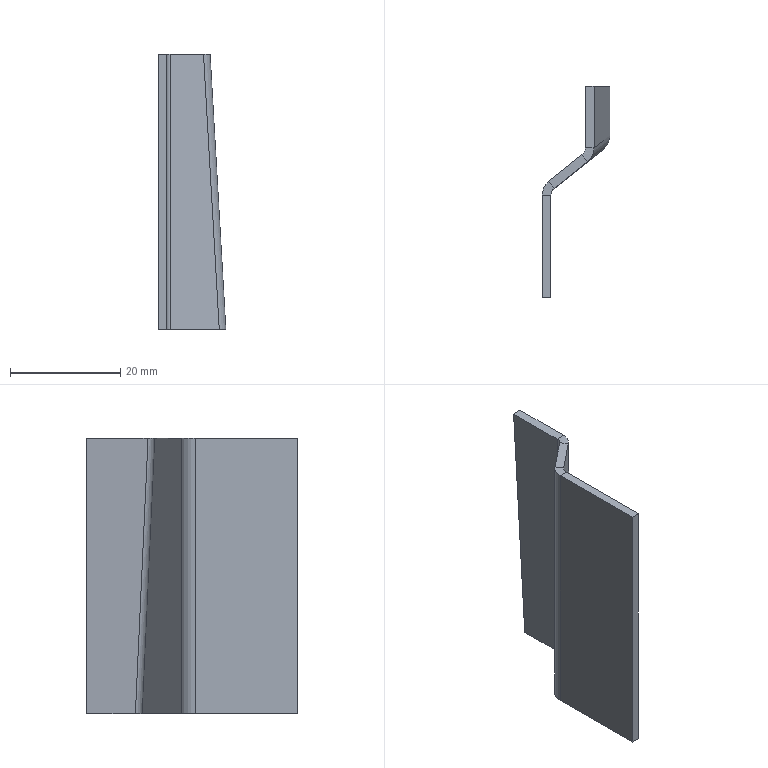Part | SolidWorks | features Fillet 2, Blend 1, FlatPattern 1, SheetMetal 1, SolidToSheetMetal 1 | 1 solid | 22 faces | box 12.3 x 38.3 x 50.091 mm | volume 3396 mm3 | plane 16 | cylinder 4 | spline 2 | commonest cylinder face diameters 3.2 x2 6.4 x2
STEP:
#1=CARTESIAN_POINT('',(9.103,38.3,-50.091));
#2=VERTEX_POINT('',#1);
#3=CARTESIAN_POINT('',(10.7,38.3,-50.));
#4=VERTEX_POINT('',#3);
#5=CARTESIAN_POINT('',(9.103,38.3,-50.091));
#6=CARTESIAN_POINT('',(9.635,38.3,-50.061));
#7=CARTESIAN_POINT('',(10.168,38.3,-50.03));
#8=CARTESIAN_POINT('',(10.7,38.3,-50.));
#9=B_SPLINE_CURVE_WITH_KNOTS('',3,(#5,#6,#7,#8),.UNSPECIFIED.,.F.,.F.,(4,4),(0.,1.),.UNSPECIFIED.);
#10=EDGE_CURVE('',#2,#4,#9,.T.);
#11=ORIENTED_EDGE('',*,*,#10,.F.);
#12=CARTESIAN_POINT('',(6.241,38.3,-0.09142));
#13=VERTEX_POINT('',#12);
#14=CARTESIAN_POINT('',(6.215,38.3,0.3557));
#15=DIRECTION('',(-0.05714,0.,0.9984));
#16=VECTOR('',#15,1000.);
#17=LINE('',#14,#16);
#18=EDGE_CURVE('',#2,#13,#17,.T.);
#19=ORIENTED_EDGE('',*,*,#18,.T.);
#20=CARTESIAN_POINT('',(7.838,38.3,0.));
#21=VERTEX_POINT('',#20);
#22=CARTESIAN_POINT('',(6.241,38.3,-0.09142));
#23=CARTESIAN_POINT('',(6.773,38.3,-0.06095));
#24=CARTESIAN_POINT('',(7.306,38.3,-0.03047));
#25=CARTESIAN_POINT('',(7.838,38.3,0.));
#26=B_SPLINE_CURVE_WITH_KNOTS('',3,(#22,#23,#24,#25),.UNSPECIFIED.,.F.,.F.,(4,4),(0.,1.),.UNSPECIFIED.);
#27=EDGE_CURVE('',#13,#21,#26,.T.);
#28=ORIENTED_EDGE('',*,*,#27,.T.);
#29=CARTESIAN_POINT('',(10.7,38.3,-50.));
#30=DIRECTION('',(-0.05714,0.,0.9984));
#31=VECTOR('',#30,1000.);
#32=LINE('',#29,#31);
#33=EDGE_CURVE('',#4,#21,#32,.T.);
#34=ORIENTED_EDGE('',*,*,#33,.F.);
#35=EDGE_LOOP('',(#11,#19,#28,#34));
#36=FACE_OUTER_BOUND('',#35,.T.);
#37=CARTESIAN_POINT('',(10.7,38.3,-50.));
#38=DIRECTION('',(0.,-1.,0.));
#39=DIRECTION('',(-0.05714,0.,0.9984));
#40=AXIS2_PLACEMENT_3D('',#37,#38,#39);
#41=PLANE('',#40);
#42=ADVANCED_FACE('',(#36),#41,.F.);
#43=ORIENTED_EDGE('',*,*,#27,.F.);
#44=CARTESIAN_POINT('',(6.241,27.138,-0.09142));
#45=VERTEX_POINT('',#44);
#46=CARTESIAN_POINT('',(6.241,27.138,-0.09142));
#47=CARTESIAN_POINT('',(6.241,30.858,-0.09142));
#48=CARTESIAN_POINT('',(6.241,34.579,-0.09142));
#49=CARTESIAN_POINT('',(6.241,38.3,-0.09142));
#50=B_SPLINE_CURVE_WITH_KNOTS('',3,(#46,#47,#48,#49),.UNSPECIFIED.,.F.,.F.,(4,4),(0.0000024,0.8789),.UNSPECIFIED.);
#51=EDGE_CURVE('',#45,#13,#50,.T.);
#52=ORIENTED_EDGE('',*,*,#51,.F.);
#53=CARTESIAN_POINT('',(7.838,27.138,0.));
#54=VERTEX_POINT('',#53);
#55=CARTESIAN_POINT('',(6.241,27.138,-0.09142));
#56=CARTESIAN_POINT('',(6.773,27.138,-0.06095));
#57=CARTESIAN_POINT('',(7.306,27.138,-0.03047));
#58=CARTESIAN_POINT('',(7.838,27.138,0.));
#59=B_SPLINE_CURVE_WITH_KNOTS('',3,(#55,#56,#57,#58),.UNSPECIFIED.,.F.,.F.,(4,4),(0.,1.),.UNSPECIFIED.);
#60=EDGE_CURVE('',#45,#54,#59,.T.);
#61=ORIENTED_EDGE('',*,*,#60,.T.);
#62=CARTESIAN_POINT('',(7.838,25.6,0.));
#63=DIRECTION('',(0.,1.,0.));
#64=VECTOR('',#63,1000.);
#65=LINE('',#62,#64);
#66=EDGE_CURVE('',#54,#21,#65,.T.);
#67=ORIENTED_EDGE('',*,*,#66,.T.);
#68=EDGE_LOOP('',(#43,#52,#61,#67));
#69=FACE_OUTER_BOUND('',#68,.T.);
#70=CARTESIAN_POINT('',(6.241,38.3,-0.09142));
#71=DIRECTION('',(0.05714,0.,-0.9984));
#72=DIRECTION('',(0.9984,0.,0.05714));
#73=AXIS2_PLACEMENT_3D('',#70,#71,#72);
#74=PLANE('',#73);
#75=ADVANCED_FACE('',(#69),#74,.F.);
#76=ORIENTED_EDGE('',*,*,#60,.F.);
#77=CARTESIAN_POINT('',(5.635,25.882,0.));
#78=VERTEX_POINT('',#77);
#79=CARTESIAN_POINT('',(5.635,25.882,0.));
#80=CARTESIAN_POINT('',(6.024,26.194,-0.03618));
#81=CARTESIAN_POINT('',(6.24,26.642,-0.06879));
#82=CARTESIAN_POINT('',(6.241,27.138,-0.09142));
#83=(BOUNDED_CURVE()B_SPLINE_CURVE(3,(#79,#80,#81,#82),.UNSPECIFIED.,.F.,.F.)B_SPLINE_CURVE_WITH_KNOTS((4,4),(1.571,2.466),.UNSPECIFIED.)CURVE()GEOMETRIC_REPRESENTATION_ITEM()RATIONAL_B_SPLINE_CURVE((1.,0.9343,0.9343,1.))REPRESENTATION_ITEM(''));
#84=EDGE_CURVE('',#78,#45,#83,.T.);
#85=ORIENTED_EDGE('',*,*,#84,.F.);
#86=CARTESIAN_POINT('',(6.638,24.635,0.));
#87=VERTEX_POINT('',#86);
#88=CARTESIAN_POINT('',(5.635,25.882,0.));
#89=CARTESIAN_POINT('',(5.97,25.466,0.));
#90=CARTESIAN_POINT('',(6.304,25.051,0.));
#91=CARTESIAN_POINT('',(6.638,24.635,0.));
#92=(BOUNDED_CURVE()B_SPLINE_CURVE(3,(#88,#89,#90,#91),.UNSPECIFIED.,.F.,.F.)B_SPLINE_CURVE_WITH_KNOTS((4,4),(0.,1.),.UNSPECIFIED.)CURVE()GEOMETRIC_REPRESENTATION_ITEM()RATIONAL_B_SPLINE_CURVE((0.5,0.5,0.5,0.5))REPRESENTATION_ITEM(''));
#93=EDGE_CURVE('',#78,#87,#92,.T.);
#94=ORIENTED_EDGE('',*,*,#93,.T.);
#95=CARTESIAN_POINT('',(6.638,24.635,0.));
#96=CARTESIAN_POINT('',(7.41,25.256,0.));
#97=CARTESIAN_POINT('',(7.838,26.149,0.));
#98=CARTESIAN_POINT('',(7.838,27.138,0.));
#99=(BOUNDED_CURVE()B_SPLINE_CURVE(3,(#95,#96,#97,#98),.UNSPECIFIED.,.F.,.F.)B_SPLINE_CURVE_WITH_KNOTS((4,4),(1.571,2.466),.UNSPECIFIED.)CURVE()GEOMETRIC_REPRESENTATION_ITEM()RATIONAL_B_SPLINE_CURVE((1.,0.9343,0.9343,1.))REPRESENTATION_ITEM(''));
#100=EDGE_CURVE('',#87,#54,#99,.T.);
#101=ORIENTED_EDGE('',*,*,#100,.T.);
#102=EDGE_LOOP('',(#76,#85,#94,#101));
#103=FACE_OUTER_BOUND('',#102,.T.);
#104=CARTESIAN_POINT('',(3.376,26.119,0.1172));
#105=CARTESIAN_POINT('',(2.961,25.786,0.07811));
#106=CARTESIAN_POINT('',(2.547,25.452,0.03906));
#107=CARTESIAN_POINT('',(2.132,25.119,0.));
#108=CARTESIAN_POINT('',(5.381,23.625,0.1172));
#109=CARTESIAN_POINT('',(5.634,22.46,0.07811));
#110=CARTESIAN_POINT('',(5.888,21.295,0.03906));
#111=CARTESIAN_POINT('',(6.142,20.131,0.));
#112=CARTESIAN_POINT('',(7.895,25.646,-0.1172));
#113=CARTESIAN_POINT('',(8.978,25.147,-0.07811));
#114=CARTESIAN_POINT('',(10.061,24.649,-0.03906));
#115=CARTESIAN_POINT('',(11.143,24.151,0.));
#116=CARTESIAN_POINT('',(5.89,28.14,-0.1172));
#117=CARTESIAN_POINT('',(6.305,28.473,-0.07811));
#118=CARTESIAN_POINT('',(6.719,28.806,-0.03906));
#119=CARTESIAN_POINT('',(7.134,29.139,0.));
#120=CARTESIAN_POINT('',(3.886,30.634,-0.1172));
#121=CARTESIAN_POINT('',(3.632,31.799,-0.07811));
#122=CARTESIAN_POINT('',(3.378,32.963,-0.03906));
#123=CARTESIAN_POINT('',(3.125,34.128,0.));
#124=CARTESIAN_POINT('',(1.371,28.613,0.1172));
#125=CARTESIAN_POINT('',(0.2884,29.111,0.07811));
#126=CARTESIAN_POINT('',(-0.7944,29.609,0.03906));
#127=CARTESIAN_POINT('',(-1.877,30.108,0.));
#128=CARTESIAN_POINT('',(3.376,26.119,0.1172));
#129=CARTESIAN_POINT('',(2.961,25.786,0.07811));
#130=CARTESIAN_POINT('',(2.547,25.452,0.03906));
#131=CARTESIAN_POINT('',(2.132,25.119,0.));
#132=(BOUNDED_SURFACE()B_SPLINE_SURFACE(3,3,((#104,#105,#106,#107),(#108,#109,#110,#111),(#112,#113,#114,#115),(#116,#117,#118,#119),(#120,#121,#122,#123),(#124,#125,#126,#127),(#128,#129,#130,#131)),.UNSPECIFIED.,.T.,.F.,.F.)B_SPLINE_SURFACE_WITH_KNOTS((4,3,4),(4,4),(0.,0.5,1.),(0.,1.),.UNSPECIFIED.)GEOMETRIC_REPRESENTATION_ITEM()RATIONAL_B_SPLINE_SURFACE(((1.,1.,1.,1.),(0.3333,0.3333,0.3333,0.3333),(0.3333,0.3333,0.3333,0.3333),(1.,1.,1.,1.),(0.3333,0.3333,0.3333,0.3333),(0.3333,0.3333,0.3333,0.3333),(1.,1.,1.,1.)))REPRESENTATION_ITEM('')SURFACE());
#133=ADVANCED_FACE('',(#103),#132,.F.);
#134=ORIENTED_EDGE('',*,*,#93,.F.);
#135=CARTESIAN_POINT('',(-0.4047,21.027,0.));
#136=VERTEX_POINT('',#135);
#137=CARTESIAN_POINT('',(-0.4047,21.027,0.));
#138=CARTESIAN_POINT('',(1.609,22.646,0.));
#139=CARTESIAN_POINT('',(3.622,24.264,0.));
#140=CARTESIAN_POINT('',(5.635,25.882,0.));
#141=B_SPLINE_CURVE_WITH_KNOTS('',3,(#137,#138,#139,#140),.UNSPECIFIED.,.F.,.F.,(4,4),(0.1532,0.9238),.UNSPECIFIED.);
#142=EDGE_CURVE('',#136,#78,#141,.T.);
#143=ORIENTED_EDGE('',*,*,#142,.F.);
#144=CARTESIAN_POINT('',(0.5976,19.78,0.));
#145=VERTEX_POINT('',#144);
#146=CARTESIAN_POINT('',(-0.4047,21.027,0.));
#147=CARTESIAN_POINT('',(-0.07059,20.612,0.));
#148=CARTESIAN_POINT('',(0.2635,20.196,0.));
#149=CARTESIAN_POINT('',(0.5976,19.78,0.));
#150=B_SPLINE_CURVE_WITH_KNOTS('',3,(#146,#147,#148,#149),.UNSPECIFIED.,.F.,.F.,(4,4),(0.,1.),.UNSPECIFIED.);
#151=EDGE_CURVE('',#136,#145,#150,.T.);
#152=ORIENTED_EDGE('',*,*,#151,.T.);
#153=CARTESIAN_POINT('',(0.,19.3,0.));
#154=DIRECTION('',(0.7794,0.6265,0.));
#155=VECTOR('',#154,1000.);
#156=LINE('',#153,#155);
#157=EDGE_CURVE('',#145,#87,#156,.T.);
#158=ORIENTED_EDGE('',*,*,#157,.T.);
#159=EDGE_LOOP('',(#134,#143,#152,#158));
#160=FACE_OUTER_BOUND('',#159,.T.);
#161=CARTESIAN_POINT('',(5.635,25.882,0.));
#162=DIRECTION('',(0.,0.,-1.));
#163=DIRECTION('',(0.6265,-0.7794,0.));
#164=AXIS2_PLACEMENT_3D('',#161,#162,#163);
#165=PLANE('',#164);
#166=ADVANCED_FACE('',(#160),#165,.F.);
#167=ORIENTED_EDGE('',*,*,#151,.F.);
#168=CARTESIAN_POINT('',(-1.6,18.533,0.));
#169=VERTEX_POINT('',#168);
#170=CARTESIAN_POINT('',(1.6,18.533,0.));
#171=DIRECTION('',(0.,0.,-1.));
#172=DIRECTION('',(-1.,0.,0.));
#173=AXIS2_PLACEMENT_3D('',#170,#171,#172);
#174=CIRCLE('',#173,3.2);
#175=EDGE_CURVE('',#169,#136,#174,.T.);
#176=ORIENTED_EDGE('',*,*,#175,.F.);
#177=CARTESIAN_POINT('',(0.,18.533,0.));
#178=VERTEX_POINT('',#177);
#179=CARTESIAN_POINT('',(-1.6,18.533,0.));
#180=CARTESIAN_POINT('',(-1.067,18.533,0.));
#181=CARTESIAN_POINT('',(-0.5333,18.533,0.));
#182=CARTESIAN_POINT('',(0.,18.533,0.));
#183=B_SPLINE_CURVE_WITH_KNOTS('',3,(#179,#180,#181,#182),.UNSPECIFIED.,.F.,.F.,(4,4),(0.,1.),.UNSPECIFIED.);
#184=EDGE_CURVE('',#169,#178,#183,.T.);
#185=ORIENTED_EDGE('',*,*,#184,.T.);
#186=CARTESIAN_POINT('',(1.6,18.533,0.));
#187=DIRECTION('',(0.,0.,-1.));
#188=DIRECTION('',(1.,0.,0.));
#189=AXIS2_PLACEMENT_3D('',#186,#187,#188);
#190=CIRCLE('',#189,1.6);
#191=EDGE_CURVE('',#178,#145,#190,.T.);
#192=ORIENTED_EDGE('',*,*,#191,.T.);
#193=EDGE_LOOP('',(#167,#176,#185,#192));
#194=FACE_OUTER_BOUND('',#193,.T.);
#195=CARTESIAN_POINT('',(1.6,18.533,0.));
#196=DIRECTION('',(0.,0.,-1.));
#197=DIRECTION('',(-1.,0.,0.));
#198=AXIS2_PLACEMENT_3D('',#195,#196,#197);
#199=PLANE('',#198);
#200=ADVANCED_FACE('',(#194),#199,.F.);
#201=ORIENTED_EDGE('',*,*,#184,.F.);
#202=CARTESIAN_POINT('',(-1.6,0.,0.));
#203=VERTEX_POINT('',#202);
#204=CARTESIAN_POINT('',(-1.6,0.,0.));
#205=CARTESIAN_POINT('',(-1.6,6.178,0.));
#206=CARTESIAN_POINT('',(-1.6,12.355,0.));
#207=CARTESIAN_POINT('',(-1.6,18.533,0.));
#208=B_SPLINE_CURVE_WITH_KNOTS('',3,(#204,#205,#206,#207),.UNSPECIFIED.,.F.,.F.,(4,4),(0.03973,1.),.UNSPECIFIED.);
#209=EDGE_CURVE('',#203,#169,#208,.T.);
#210=ORIENTED_EDGE('',*,*,#209,.F.);
#211=CARTESIAN_POINT('',(0.,0.,0.));
#212=VERTEX_POINT('',#211);
#213=CARTESIAN_POINT('',(-1.6,0.,0.));
#214=CARTESIAN_POINT('',(-1.067,0.,0.));
#215=CARTESIAN_POINT('',(-0.5333,0.,0.));
#216=CARTESIAN_POINT('',(0.,0.,0.));
#217=B_SPLINE_CURVE_WITH_KNOTS('',3,(#213,#214,#215,#216),.UNSPECIFIED.,.F.,.F.,(4,4),(0.,1.),.UNSPECIFIED.);
#218=EDGE_CURVE('',#203,#212,#217,.T.);
#219=ORIENTED_EDGE('',*,*,#218,.T.);
#220=CARTESIAN_POINT('',(0.,19.3,0.));
#221=DIRECTION('',(0.,1.,0.));
#222=VECTOR('',#221,1000.);
#223=LINE('',#220,#222);
#224=EDGE_CURVE('',#212,#178,#223,.T.);
#225=ORIENTED_EDGE('',*,*,#224,.T.);
#226=EDGE_LOOP('',(#201,#210,#219,#225));
#227=FACE_OUTER_BOUND('',#226,.T.);
#228=CARTESIAN_POINT('',(-1.6,18.533,0.));
#229=DIRECTION('',(0.,0.,-1.));
#230=DIRECTION('',(1.,0.,0.));
#231=AXIS2_PLACEMENT_3D('',#228,#229,#230);
#232=PLANE('',#231);
#233=ADVANCED_FACE('',(#227),#232,.F.);
#234=ORIENTED_EDGE('',*,*,#218,.F.);
#235=CARTESIAN_POINT('',(-1.6,0.,-50.));
#236=VERTEX_POINT('',#235);
#237=CARTESIAN_POINT('',(-1.6,0.,0.));
#238=DIRECTION('',(0.,0.,1.));
#239=VECTOR('',#238,1000.);
#240=LINE('',#237,#239);
#241=EDGE_CURVE('',#236,#203,#240,.T.);
#242=ORIENTED_EDGE('',*,*,#241,.F.);
#243=CARTESIAN_POINT('',(0.,0.,-50.));
#244=VERTEX_POINT('',#243);
#245=CARTESIAN_POINT('',(-1.6,0.,-50.));
#246=CARTESIAN_POINT('',(-1.067,0.,-50.));
#247=CARTESIAN_POINT('',(-0.5333,0.,-50.));
#248=CARTESIAN_POINT('',(0.,0.,-50.));
#249=B_SPLINE_CURVE_WITH_KNOTS('',3,(#245,#246,#247,#248),.UNSPECIFIED.,.F.,.F.,(4,4),(0.,1.),.UNSPECIFIED.);
#250=EDGE_CURVE('',#236,#244,#249,.T.);
#251=ORIENTED_EDGE('',*,*,#250,.T.);
#252=CARTESIAN_POINT('',(0.,0.,-50.));
#253=DIRECTION('',(0.,0.,1.));
#254=VECTOR('',#253,1000.);
#255=LINE('',#252,#254);
#256=EDGE_CURVE('',#244,#212,#255,.T.);
#257=ORIENTED_EDGE('',*,*,#256,.T.);
#258=EDGE_LOOP('',(#234,#242,#251,#257));
#259=FACE_OUTER_BOUND('',#258,.T.);
#260=CARTESIAN_POINT('',(0.,0.,-50.));
#261=DIRECTION('',(0.,-1.,0.));
#262=DIRECTION('',(0.,0.,1.));
#263=AXIS2_PLACEMENT_3D('',#260,#261,#262);
#264=PLANE('',#263);
#265=ADVANCED_FACE('',(#259),#264,.T.);
#266=ORIENTED_EDGE('',*,*,#250,.F.);
#267=CARTESIAN_POINT('',(-1.6,18.533,-50.));
#268=VERTEX_POINT('',#267);
#269=CARTESIAN_POINT('',(-1.6,0.,-50.));
#270=CARTESIAN_POINT('',(-1.6,6.178,-50.));
#271=CARTESIAN_POINT('',(-1.6,12.355,-50.));
#272=CARTESIAN_POINT('',(-1.6,18.533,-50.));
#273=B_SPLINE_CURVE_WITH_KNOTS('',3,(#269,#270,#271,#272),.UNSPECIFIED.,.F.,.F.,(4,4),(0.,1.),.UNSPECIFIED.);
#274=EDGE_CURVE('',#236,#268,#273,.T.);
#275=ORIENTED_EDGE('',*,*,#274,.T.);
#276=CARTESIAN_POINT('',(0.,18.533,-50.));
#277=VERTEX_POINT('',#276);
#278=CARTESIAN_POINT('',(-1.6,18.533,-50.));
#279=CARTESIAN_POINT('',(-1.067,18.533,-50.));
#280=CARTESIAN_POINT('',(-0.5333,18.533,-50.));
#281=CARTESIAN_POINT('',(0.,18.533,-50.));
#282=B_SPLINE_CURVE_WITH_KNOTS('',3,(#278,#279,#280,#281),.UNSPECIFIED.,.F.,.F.,(4,4),(0.,1.),.UNSPECIFIED.);
#283=EDGE_CURVE('',#268,#277,#282,.T.);
#284=ORIENTED_EDGE('',*,*,#283,.T.);
#285=CARTESIAN_POINT('',(0.,0.,-50.));
#286=DIRECTION('',(0.,1.,0.));
#287=VECTOR('',#286,1000.);
#288=LINE('',#285,#287);
#289=EDGE_CURVE('',#244,#277,#288,.T.);
#290=ORIENTED_EDGE('',*,*,#289,.F.);
#291=EDGE_LOOP('',(#266,#275,#284,#290));
#292=FACE_OUTER_BOUND('',#291,.T.);
#293=CARTESIAN_POINT('',(-1.6,0.,-50.));
#294=DIRECTION('',(0.,0.,1.));
#295=DIRECTION('',(1.,0.,0.));
#296=AXIS2_PLACEMENT_3D('',#293,#294,#295);
#297=PLANE('',#296);
#298=ADVANCED_FACE('',(#292),#297,.F.);
#299=ORIENTED_EDGE('',*,*,#283,.F.);
#300=CARTESIAN_POINT('',(-0.4047,21.027,-50.));
#301=VERTEX_POINT('',#300);
#302=CARTESIAN_POINT('',(1.6,18.533,-50.));
#303=DIRECTION('',(0.,0.,1.));
#304=DIRECTION('',(-1.,0.,0.));
#305=AXIS2_PLACEMENT_3D('',#302,#303,#304);
#306=CIRCLE('',#305,3.2);
#307=EDGE_CURVE('',#301,#268,#306,.T.);
#308=ORIENTED_EDGE('',*,*,#307,.F.);
#309=CARTESIAN_POINT('',(0.5976,19.78,-50.));
#310=VERTEX_POINT('',#309);
#311=CARTESIAN_POINT('',(-0.4047,21.027,-50.));
#312=CARTESIAN_POINT('',(-0.07059,20.612,-50.));
#313=CARTESIAN_POINT('',(0.2635,20.196,-50.));
#314=CARTESIAN_POINT('',(0.5976,19.78,-50.));
#315=B_SPLINE_CURVE_WITH_KNOTS('',3,(#311,#312,#313,#314),.UNSPECIFIED.,.F.,.F.,(4,4),(0.,1.),.UNSPECIFIED.);
#316=EDGE_CURVE('',#301,#310,#315,.T.);
#317=ORIENTED_EDGE('',*,*,#316,.T.);
#318=CARTESIAN_POINT('',(1.6,18.533,-50.));
#319=DIRECTION('',(0.,0.,1.));
#320=DIRECTION('',(1.,0.,0.));
#321=AXIS2_PLACEMENT_3D('',#318,#319,#320);
#322=CIRCLE('',#321,1.6);
#323=EDGE_CURVE('',#310,#277,#322,.T.);
#324=ORIENTED_EDGE('',*,*,#323,.T.);
#325=EDGE_LOOP('',(#299,#308,#317,#324));
#326=FACE_OUTER_BOUND('',#325,.T.);
#327=CARTESIAN_POINT('',(1.6,18.533,-50.));
#328=DIRECTION('',(0.,0.,-1.));
#329=DIRECTION('',(-1.,0.,0.));
#330=AXIS2_PLACEMENT_3D('',#327,#328,#329);
#331=PLANE('',#330);
#332=ADVANCED_FACE('',(#326),#331,.T.);
#333=ORIENTED_EDGE('',*,*,#316,.F.);
#334=CARTESIAN_POINT('',(8.497,28.182,-50.));
#335=VERTEX_POINT('',#334);
#336=CARTESIAN_POINT('',(-0.4047,21.027,-50.));
#337=CARTESIAN_POINT('',(2.563,23.412,-50.));
#338=CARTESIAN_POINT('',(5.53,25.797,-50.));
#339=CARTESIAN_POINT('',(8.497,28.182,-50.));
#340=B_SPLINE_CURVE_WITH_KNOTS('',3,(#336,#337,#338,#339),.UNSPECIFIED.,.F.,.F.,(4,4),(0.,1.),.UNSPECIFIED.);
#341=EDGE_CURVE('',#301,#335,#340,.T.);
#342=ORIENTED_EDGE('',*,*,#341,.T.);
#343=CARTESIAN_POINT('',(9.499,26.935,-50.));
#344=VERTEX_POINT('',#343);
#345=CARTESIAN_POINT('',(8.497,28.182,-50.));
#346=CARTESIAN_POINT('',(8.831,27.766,-50.));
#347=CARTESIAN_POINT('',(9.165,27.351,-50.));
#348=CARTESIAN_POINT('',(9.499,26.935,-50.));
#349=B_SPLINE_CURVE_WITH_KNOTS('',3,(#345,#346,#347,#348),.UNSPECIFIED.,.F.,.F.,(4,4),(0.,1.),.UNSPECIFIED.);
#350=EDGE_CURVE('',#335,#344,#349,.T.);
#351=ORIENTED_EDGE('',*,*,#350,.T.);
#352=CARTESIAN_POINT('',(0.,19.3,-50.));
#353=DIRECTION('',(0.7794,0.6265,0.));
#354=VECTOR('',#353,1000.);
#355=LINE('',#352,#354);
#356=EDGE_CURVE('',#310,#344,#355,.T.);
#357=ORIENTED_EDGE('',*,*,#356,.F.);
#358=EDGE_LOOP('',(#333,#342,#351,#357));
#359=FACE_OUTER_BOUND('',#358,.T.);
#360=CARTESIAN_POINT('',(-0.4047,21.027,-50.));
#361=DIRECTION('',(0.,0.,1.));
#362=DIRECTION('',(0.6265,-0.7794,0.));
#363=AXIS2_PLACEMENT_3D('',#360,#361,#362);
#364=PLANE('',#363);
#365=ADVANCED_FACE('',(#359),#364,.F.);
#366=ORIENTED_EDGE('',*,*,#350,.F.);
#367=CARTESIAN_POINT('',(9.103,29.438,-50.091));
#368=VERTEX_POINT('',#367);
#369=CARTESIAN_POINT('',(9.103,29.438,-50.091));
#370=CARTESIAN_POINT('',(9.101,28.942,-50.069));
#371=CARTESIAN_POINT('',(8.885,28.494,-50.036));
#372=CARTESIAN_POINT('',(8.497,28.182,-50.));
#373=(BOUNDED_CURVE()B_SPLINE_CURVE(3,(#369,#370,#371,#372),.UNSPECIFIED.,.F.,.F.)B_SPLINE_CURVE_WITH_KNOTS((4,4),(3.817,4.712),.UNSPECIFIED.)CURVE()GEOMETRIC_REPRESENTATION_ITEM()RATIONAL_B_SPLINE_CURVE((1.,0.9343,0.9343,1.))REPRESENTATION_ITEM(''));
#374=EDGE_CURVE('',#368,#335,#373,.T.);
#375=ORIENTED_EDGE('',*,*,#374,.F.);
#376=CARTESIAN_POINT('',(10.7,29.438,-50.));
#377=VERTEX_POINT('',#376);
#378=CARTESIAN_POINT('',(9.103,29.438,-50.091));
#379=CARTESIAN_POINT('',(9.635,29.438,-50.061));
#380=CARTESIAN_POINT('',(10.168,29.438,-50.03));
#381=CARTESIAN_POINT('',(10.7,29.438,-50.));
#382=(BOUNDED_CURVE()B_SPLINE_CURVE(3,(#378,#379,#380,#381),.UNSPECIFIED.,.F.,.F.)B_SPLINE_CURVE_WITH_KNOTS((4,4),(0.,1.),.UNSPECIFIED.)CURVE()GEOMETRIC_REPRESENTATION_ITEM()RATIONAL_B_SPLINE_CURVE((0.6152,0.6152,0.6152,0.6152))REPRESENTATION_ITEM(''));
#383=EDGE_CURVE('',#368,#377,#382,.T.);
#384=ORIENTED_EDGE('',*,*,#383,.T.);
#385=CARTESIAN_POINT('',(10.7,29.438,-50.));
#386=CARTESIAN_POINT('',(10.7,28.449,-50.));
#387=CARTESIAN_POINT('',(10.272,27.556,-50.));
#388=CARTESIAN_POINT('',(9.499,26.935,-50.));
#389=(BOUNDED_CURVE()B_SPLINE_CURVE(3,(#385,#386,#387,#388),.UNSPECIFIED.,.F.,.F.)B_SPLINE_CURVE_WITH_KNOTS((4,4),(3.817,4.712),.UNSPECIFIED.)CURVE()GEOMETRIC_REPRESENTATION_ITEM()RATIONAL_B_SPLINE_CURVE((1.,0.9343,0.9343,1.))REPRESENTATION_ITEM(''));
#390=EDGE_CURVE('',#377,#344,#389,.T.);
#391=ORIENTED_EDGE('',*,*,#390,.T.);
#392=EDGE_LOOP('',(#366,#375,#384,#391));
#393=FACE_OUTER_BOUND('',#392,.T.);
#394=CARTESIAN_POINT('',(4.994,27.419,-50.));
#395=CARTESIAN_POINT('',(5.408,27.752,-49.961));
#396=CARTESIAN_POINT('',(5.823,28.086,-49.922));
#397=CARTESIAN_POINT('',(6.238,28.419,-49.883));
#398=CARTESIAN_POINT('',(0.9844,32.408,-50.));
#399=CARTESIAN_POINT('',(2.067,31.909,-49.961));
#400=CARTESIAN_POINT('',(3.15,31.411,-49.922));
#401=CARTESIAN_POINT('',(4.233,30.913,-49.883));
#402=CARTESIAN_POINT('',(5.986,36.428,-50.));
#403=CARTESIAN_POINT('',(6.24,35.263,-50.039));
#404=CARTESIAN_POINT('',(6.494,34.099,-50.078));
#405=CARTESIAN_POINT('',(6.747,32.934,-50.117));
#406=CARTESIAN_POINT('',(9.996,31.439,-50.));
#407=CARTESIAN_POINT('',(9.581,31.106,-50.039));
#408=CARTESIAN_POINT('',(9.167,30.773,-50.078));
#409=CARTESIAN_POINT('',(8.752,30.44,-50.117));
#410=CARTESIAN_POINT('',(14.005,26.451,-50.));
#411=CARTESIAN_POINT('',(12.922,26.949,-50.039));
#412=CARTESIAN_POINT('',(11.839,27.447,-50.078));
#413=CARTESIAN_POINT('',(10.757,27.946,-50.117));
#414=CARTESIAN_POINT('',(9.003,22.431,-50.));
#415=CARTESIAN_POINT('',(8.75,23.595,-49.961));
#416=CARTESIAN_POINT('',(8.496,24.76,-49.922));
#417=CARTESIAN_POINT('',(8.242,25.925,-49.883));
#418=CARTESIAN_POINT('',(4.994,27.419,-50.));
#419=CARTESIAN_POINT('',(5.408,27.752,-49.961));
#420=CARTESIAN_POINT('',(5.823,28.086,-49.922));
#421=CARTESIAN_POINT('',(6.238,28.419,-49.883));
#422=(BOUNDED_SURFACE()B_SPLINE_SURFACE(3,3,((#394,#395,#396,#397),(#398,#399,#400,#401),(#402,#403,#404,#405),(#406,#407,#408,#409),(#410,#411,#412,#413),(#414,#415,#416,#417),(#418,#419,#420,#421)),.UNSPECIFIED.,.T.,.F.,.F.)B_SPLINE_SURFACE_WITH_KNOTS((4,3,4),(4,4),(0.,0.5,1.),(0.,1.),.UNSPECIFIED.)GEOMETRIC_REPRESENTATION_ITEM()RATIONAL_B_SPLINE_SURFACE(((1.,1.,1.,1.),(0.3333,0.3333,0.3333,0.3333),(0.3333,0.3333,0.3333,0.3333),(1.,1.,1.,1.),(0.3333,0.3333,0.3333,0.3333),(0.3333,0.3333,0.3333,0.3333),(1.,1.,1.,1.)))REPRESENTATION_ITEM('')SURFACE());
#423=ADVANCED_FACE('',(#393),#422,.T.);
#424=CARTESIAN_POINT('',(9.103,29.438,-50.091));
#425=CARTESIAN_POINT('',(9.103,32.392,-50.091));
#426=CARTESIAN_POINT('',(9.103,35.346,-50.091));
#427=CARTESIAN_POINT('',(9.103,38.3,-50.091));
#428=B_SPLINE_CURVE_WITH_KNOTS('',3,(#424,#425,#426,#427),.UNSPECIFIED.,.F.,.F.,(4,4),(0.,1.),.UNSPECIFIED.);
#429=EDGE_CURVE('',#368,#2,#428,.T.);
#430=ORIENTED_EDGE('',*,*,#429,.T.);
#431=ORIENTED_EDGE('',*,*,#10,.T.);
#432=CARTESIAN_POINT('',(10.7,38.3,-50.));
#433=DIRECTION('',(0.,1.,0.));
#434=VECTOR('',#433,1000.);
#435=LINE('',#432,#434);
#436=EDGE_CURVE('',#377,#4,#435,.T.);
#437=ORIENTED_EDGE('',*,*,#436,.F.);
#438=ORIENTED_EDGE('',*,*,#383,.F.);
#439=EDGE_LOOP('',(#430,#431,#437,#438));
#440=FACE_OUTER_BOUND('',#439,.T.);
#441=CARTESIAN_POINT('',(9.103,29.438,-50.091));
#442=DIRECTION('',(-0.05714,0.,0.9984));
#443=DIRECTION('',(0.9984,0.,0.05714));
#444=AXIS2_PLACEMENT_3D('',#441,#442,#443);
#445=PLANE('',#444);
#446=ADVANCED_FACE('',(#440),#445,.F.);
#447=ORIENTED_EDGE('',*,*,#390,.F.);
#448=CARTESIAN_POINT('',(7.742,27.06,1.688));
#449=DIRECTION('',(0.05708,0.04588,-0.9973));
#450=VECTOR('',#449,1000.);
#451=LINE('',#448,#450);
#452=EDGE_CURVE('',#54,#377,#451,.T.);
#453=ORIENTED_EDGE('',*,*,#452,.F.);
#454=ORIENTED_EDGE('',*,*,#100,.F.);
#455=CARTESIAN_POINT('',(6.552,24.566,1.505));
#456=DIRECTION('',(-0.05708,-0.04588,0.9973));
#457=VECTOR('',#456,1000.);
#458=LINE('',#455,#457);
#459=EDGE_CURVE('',#344,#87,#458,.T.);
#460=ORIENTED_EDGE('',*,*,#459,.F.);
#461=EDGE_LOOP('',(#447,#453,#454,#460));
#462=FACE_OUTER_BOUND('',#461,.T.);
#463=CARTESIAN_POINT('',(4.547,27.06,1.505));
#464=DIRECTION('',(-0.05708,-0.04588,0.9973));
#465=DIRECTION('',(0.9984,0.,0.05714));
#466=AXIS2_PLACEMENT_3D('',#463,#464,#465);
#467=CYLINDRICAL_SURFACE('',#466,3.2);
#468=ADVANCED_FACE('',(#462),#467,.T.);
#469=ORIENTED_EDGE('',*,*,#66,.F.);
#470=ORIENTED_EDGE('',*,*,#452,.T.);
#471=ORIENTED_EDGE('',*,*,#436,.T.);
#472=ORIENTED_EDGE('',*,*,#33,.T.);
#473=EDGE_LOOP('',(#469,#470,#471,#472));
#474=FACE_OUTER_BOUND('',#473,.T.);
#475=CARTESIAN_POINT('',(7.813,0.,0.4471));
#476=DIRECTION('',(-0.9984,0.,-0.05714));
#477=DIRECTION('',(-0.05714,0.,0.9984));
#478=AXIS2_PLACEMENT_3D('',#475,#476,#477);
#479=PLANE('',#478);
#480=ADVANCED_FACE('',(#474),#479,.F.);
#481=ORIENTED_EDGE('',*,*,#323,.F.);
#482=CARTESIAN_POINT('',(0.5976,19.78,-50.));
#483=DIRECTION('',(0.,0.,-1.));
#484=VECTOR('',#483,1000.);
#485=LINE('',#482,#484);
#486=EDGE_CURVE('',#145,#310,#485,.T.);
#487=ORIENTED_EDGE('',*,*,#486,.F.);
#488=ORIENTED_EDGE('',*,*,#191,.F.);
#489=CARTESIAN_POINT('',(0.,18.533,0.));
#490=DIRECTION('',(0.,0.,1.));
#491=VECTOR('',#490,1000.);
#492=LINE('',#489,#491);
#493=EDGE_CURVE('',#277,#178,#492,.T.);
#494=ORIENTED_EDGE('',*,*,#493,.F.);
#495=EDGE_LOOP('',(#481,#487,#488,#494));
#496=FACE_OUTER_BOUND('',#495,.T.);
#497=CARTESIAN_POINT('',(1.6,18.533,0.));
#498=DIRECTION('',(0.,0.,-1.));
#499=DIRECTION('',(-1.,0.,0.));
#500=AXIS2_PLACEMENT_3D('',#497,#498,#499);
#501=CYLINDRICAL_SURFACE('',#500,1.6);
#502=ADVANCED_FACE('',(#496),#501,.F.);
#503=ORIENTED_EDGE('',*,*,#289,.T.);
#504=ORIENTED_EDGE('',*,*,#493,.T.);
#505=ORIENTED_EDGE('',*,*,#224,.F.);
#506=ORIENTED_EDGE('',*,*,#256,.F.);
#507=EDGE_LOOP('',(#503,#504,#505,#506));
#508=FACE_OUTER_BOUND('',#507,.T.);
#509=CARTESIAN_POINT('',(0.,0.,0.));
#510=DIRECTION('',(-1.,0.,0.));
#511=DIRECTION('',(0.,-1.,0.));
#512=AXIS2_PLACEMENT_3D('',#509,#510,#511);
#513=PLANE('',#512);
#514=ADVANCED_FACE('',(#508),#513,.F.);
#515=ORIENTED_EDGE('',*,*,#356,.T.);
#516=ORIENTED_EDGE('',*,*,#459,.T.);
#517=ORIENTED_EDGE('',*,*,#157,.F.);
#518=ORIENTED_EDGE('',*,*,#486,.T.);
#519=EDGE_LOOP('',(#515,#516,#517,#518));
#520=FACE_OUTER_BOUND('',#519,.T.);
#521=CARTESIAN_POINT('',(-9.424,11.725,0.));
#522=DIRECTION('',(-0.6265,0.7794,0.));
#523=DIRECTION('',(-0.7794,-0.6265,0.));
#524=AXIS2_PLACEMENT_3D('',#521,#522,#523);
#525=PLANE('',#524);
#526=ADVANCED_FACE('',(#520),#525,.F.);
#527=ORIENTED_EDGE('',*,*,#374,.T.);
#528=CARTESIAN_POINT('',(5.549,25.813,1.505));
#529=DIRECTION('',(-0.05708,-0.04588,0.9973));
#530=VECTOR('',#529,1000.);
#531=LINE('',#528,#530);
#532=EDGE_CURVE('',#335,#78,#531,.T.);
#533=ORIENTED_EDGE('',*,*,#532,.T.);
#534=ORIENTED_EDGE('',*,*,#84,.T.);
#535=CARTESIAN_POINT('',(6.144,27.06,1.596));
#536=DIRECTION('',(0.05708,0.04588,-0.9973));
#537=VECTOR('',#536,1000.);
#538=LINE('',#535,#537);
#539=EDGE_CURVE('',#45,#368,#538,.T.);
#540=ORIENTED_EDGE('',*,*,#539,.T.);
#541=EDGE_LOOP('',(#527,#533,#534,#540));
#542=FACE_OUTER_BOUND('',#541,.T.);
#543=CARTESIAN_POINT('',(4.547,27.06,1.505));
#544=DIRECTION('',(-0.05708,-0.04588,0.9973));
#545=DIRECTION('',(0.9984,0.,0.05714));
#546=AXIS2_PLACEMENT_3D('',#543,#544,#545);
#547=CYLINDRICAL_SURFACE('',#546,1.6);
#548=ADVANCED_FACE('',(#542),#547,.F.);
#549=ORIENTED_EDGE('',*,*,#51,.T.);
#550=ORIENTED_EDGE('',*,*,#18,.F.);
#551=ORIENTED_EDGE('',*,*,#429,.F.);
#552=ORIENTED_EDGE('',*,*,#539,.F.);
#553=EDGE_LOOP('',(#549,#550,#551,#552));
#554=FACE_OUTER_BOUND('',#553,.T.);
#555=CARTESIAN_POINT('',(6.215,0.,0.3557));
#556=DIRECTION('',(-0.9984,0.,-0.05714));
#557=DIRECTION('',(-0.05714,0.,0.9984));
#558=AXIS2_PLACEMENT_3D('',#555,#556,#557);
#559=PLANE('',#558);
#560=ADVANCED_FACE('',(#554),#559,.T.);
#561=ORIENTED_EDGE('',*,*,#307,.T.);
#562=CARTESIAN_POINT('',(-1.6,18.533,0.));
#563=DIRECTION('',(0.,0.,1.));
#564=VECTOR('',#563,1000.);
#565=LINE('',#562,#564);
#566=EDGE_CURVE('',#268,#169,#565,.T.);
#567=ORIENTED_EDGE('',*,*,#566,.T.);
#568=ORIENTED_EDGE('',*,*,#175,.T.);
#569=CARTESIAN_POINT('',(-0.4047,21.027,0.));
#570=DIRECTION('',(0.,0.,-1.));
#571=VECTOR('',#570,1000.);
#572=LINE('',#569,#571);
#573=EDGE_CURVE('',#136,#301,#572,.T.);
#574=ORIENTED_EDGE('',*,*,#573,.T.);
#575=EDGE_LOOP('',(#561,#567,#568,#574));
#576=FACE_OUTER_BOUND('',#575,.T.);
#577=CARTESIAN_POINT('',(1.6,18.533,0.));
#578=DIRECTION('',(0.,0.,-1.));
#579=DIRECTION('',(-1.,0.,0.));
#580=AXIS2_PLACEMENT_3D('',#577,#578,#579);
#581=CYLINDRICAL_SURFACE('',#580,3.2);
#582=ADVANCED_FACE('',(#576),#581,.T.);
#583=ORIENTED_EDGE('',*,*,#274,.F.);
#584=ORIENTED_EDGE('',*,*,#241,.T.);
#585=ORIENTED_EDGE('',*,*,#209,.T.);
#586=ORIENTED_EDGE('',*,*,#566,.F.);
#587=EDGE_LOOP('',(#583,#584,#585,#586));
#588=FACE_OUTER_BOUND('',#587,.T.);
#589=CARTESIAN_POINT('',(-1.6,0.,0.));
#590=DIRECTION('',(-1.,0.,0.));
#591=DIRECTION('',(0.,-1.,0.));
#592=AXIS2_PLACEMENT_3D('',#589,#590,#591);
#593=PLANE('',#592);
#594=ADVANCED_FACE('',(#588),#593,.T.);
#595=ORIENTED_EDGE('',*,*,#341,.F.);
#596=ORIENTED_EDGE('',*,*,#573,.F.);
#597=ORIENTED_EDGE('',*,*,#142,.T.);
#598=ORIENTED_EDGE('',*,*,#532,.F.);
#599=EDGE_LOOP('',(#595,#596,#597,#598));
#600=FACE_OUTER_BOUND('',#599,.T.);
#601=CARTESIAN_POINT('',(-10.427,12.973,0.));
#602=DIRECTION('',(-0.6265,0.7794,0.));
#603=DIRECTION('',(-0.7794,-0.6265,0.));
#604=AXIS2_PLACEMENT_3D('',#601,#602,#603);
#605=PLANE('',#604);
#606=ADVANCED_FACE('',(#600),#605,.T.);
#607=CLOSED_SHELL('',(#42,#75,#133,#166,#200,#233,#265,#298,#332,#365,#423,#446,#468,#480,#502,#514,#526,#548,#560,#582,#594,#606));
#608=MANIFOLD_SOLID_BREP('',#607);
#609=CARTESIAN_POINT('',(0.,0.,0.));
#610=DIRECTION('',(0.,0.,1.));
#611=DIRECTION('',(1.,0.,0.));
#612=AXIS2_PLACEMENT_3D('',#609,#610,#611);
#613=(LENGTH_UNIT()NAMED_UNIT(*)SI_UNIT(.MILLI.,.METRE.));
#614=UNCERTAINTY_MEASURE_WITH_UNIT(LENGTH_MEASURE(0.00001),#613,'','');
#615=(NAMED_UNIT(*)PLANE_ANGLE_UNIT()SI_UNIT($,.RADIAN.));
#616=(NAMED_UNIT(*)SI_UNIT($,.STERADIAN.)SOLID_ANGLE_UNIT());
#617=(GEOMETRIC_REPRESENTATION_CONTEXT(3)GLOBAL_UNCERTAINTY_ASSIGNED_CONTEXT((#614))GLOBAL_UNIT_ASSIGNED_CONTEXT((#613,#615,#616))REPRESENTATION_CONTEXT('',''));
#618=ADVANCED_BREP_SHAPE_REPRESENTATION('',(#608,#612),#617);